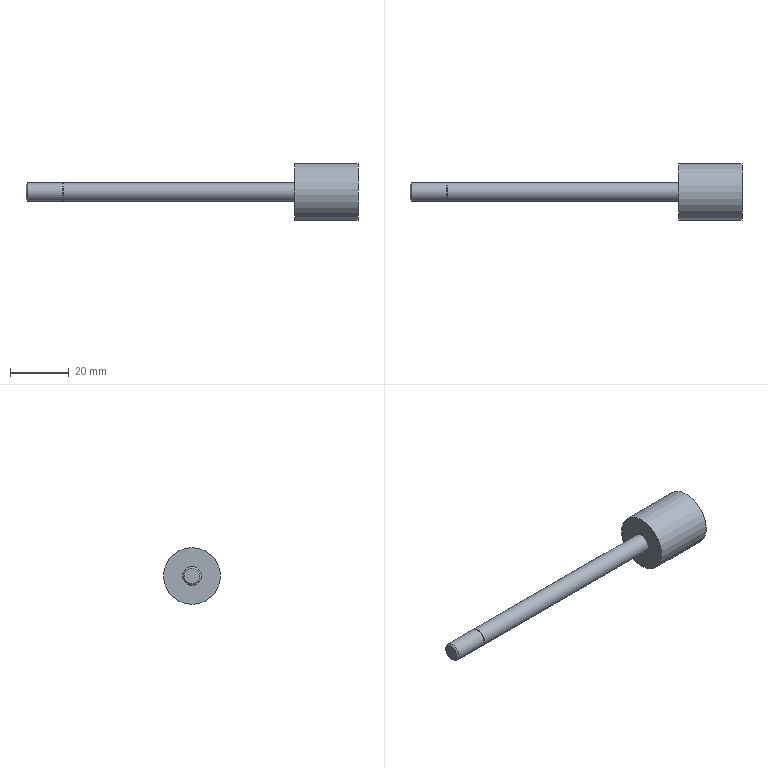Part | NX | features solid 2 | 1 solid | 10 faces | box 112.725 x 19.241 x 19.241 mm | volume 9120 mm3 | plane 5 | cylinder 4 | cone 1 | commonest cylinder face diameters 6.35 x2 5.842 x1 19.241 x1
STEP:
#1=CARTESIAN_POINT('',(78.588,0.,3.175));
#2=VERTEX_POINT('',#1);
#3=CARTESIAN_POINT('',(78.588,0.,0.));
#4=DIRECTION('',(-1.,0.,0.));
#5=DIRECTION('',(0.,0.,1.));
#6=AXIS2_PLACEMENT_3D('',#3,#4,#5);
#7=CIRCLE('',#6,3.175);
#8=EDGE_CURVE('',#2,#2,#7,.T.);
#9=ORIENTED_EDGE('',*,*,#8,.T.);
#10=EDGE_LOOP('',(#9));
#11=FACE_BOUND('',#10,.T.);
#12=CARTESIAN_POINT('',(0.,0.,3.175));
#13=VERTEX_POINT('',#12);
#14=CARTESIAN_POINT('',(0.,0.,0.));
#15=DIRECTION('',(-1.,0.,0.));
#16=DIRECTION('',(0.,0.,1.));
#17=AXIS2_PLACEMENT_3D('',#14,#15,#16);
#18=CIRCLE('',#17,3.175);
#19=EDGE_CURVE('',#13,#13,#18,.F.);
#20=ORIENTED_EDGE('',*,*,#19,.T.);
#21=EDGE_LOOP('',(#20));
#22=FACE_BOUND('',#21,.T.);
#23=CARTESIAN_POINT('',(100.025,0.,0.));
#24=DIRECTION('',(-1.,0.,0.));
#25=DIRECTION('',(0.,0.,1.));
#26=AXIS2_PLACEMENT_3D('',#23,#24,#25);
#27=CYLINDRICAL_SURFACE('',#26,3.175);
#28=ADVANCED_FACE('',(#11,#22),#27,.T.);
#29=CARTESIAN_POINT('',(78.588,0.,9.62));
#30=VERTEX_POINT('',#29);
#31=CARTESIAN_POINT('',(78.588,0.,0.));
#32=DIRECTION('',(-1.,0.,0.));
#33=DIRECTION('',(0.,0.,1.));
#34=AXIS2_PLACEMENT_3D('',#31,#32,#33);
#35=CIRCLE('',#34,9.62);
#36=EDGE_CURVE('',#30,#30,#35,.T.);
#37=ORIENTED_EDGE('',*,*,#36,.T.);
#38=EDGE_LOOP('',(#37));
#39=FACE_BOUND('',#38,.T.);
#40=ORIENTED_EDGE('',*,*,#8,.F.);
#41=EDGE_LOOP('',(#40));
#42=FACE_BOUND('',#41,.T.);
#43=CARTESIAN_POINT('',(78.588,3.175,0.));
#44=DIRECTION('',(-1.,0.,0.));
#45=DIRECTION('',(0.,0.,1.));
#46=AXIS2_PLACEMENT_3D('',#43,#44,#45);
#47=PLANE('',#46);
#48=ADVANCED_FACE('',(#39,#42),#47,.T.);
#49=CARTESIAN_POINT('',(100.025,0.,9.62));
#50=VERTEX_POINT('',#49);
#51=CARTESIAN_POINT('',(100.025,0.,0.));
#52=DIRECTION('',(-1.,0.,0.));
#53=DIRECTION('',(0.,0.,1.));
#54=AXIS2_PLACEMENT_3D('',#51,#52,#53);
#55=CIRCLE('',#54,9.62);
#56=EDGE_CURVE('',#50,#50,#55,.T.);
#57=ORIENTED_EDGE('',*,*,#56,.T.);
#58=EDGE_LOOP('',(#57));
#59=FACE_BOUND('',#58,.T.);
#60=ORIENTED_EDGE('',*,*,#36,.F.);
#61=EDGE_LOOP('',(#60));
#62=FACE_BOUND('',#61,.T.);
#63=CARTESIAN_POINT('',(100.025,0.,0.));
#64=DIRECTION('',(-1.,0.,0.));
#65=DIRECTION('',(0.,0.,1.));
#66=AXIS2_PLACEMENT_3D('',#63,#64,#65);
#67=CYLINDRICAL_SURFACE('',#66,9.62);
#68=ADVANCED_FACE('',(#59,#62),#67,.T.);
#69=ORIENTED_EDGE('',*,*,#56,.F.);
#70=EDGE_LOOP('',(#69));
#71=FACE_BOUND('',#70,.T.);
#72=CARTESIAN_POINT('',(100.025,9.62,0.));
#73=DIRECTION('',(1.,0.,0.));
#74=DIRECTION('',(0.,0.,-1.));
#75=AXIS2_PLACEMENT_3D('',#72,#73,#74);
#76=PLANE('',#75);
#77=ADVANCED_FACE('',(#71),#76,.T.);
#78=CARTESIAN_POINT('',(-0.254,0.,-3.175));
#79=VERTEX_POINT('',#78);
#80=CARTESIAN_POINT('',(-0.254,0.,0.));
#81=DIRECTION('',(1.,0.,0.));
#82=DIRECTION('',(0.,0.,-1.));
#83=AXIS2_PLACEMENT_3D('',#80,#81,#82);
#84=CIRCLE('',#83,3.175);
#85=EDGE_CURVE('',#79,#79,#84,.F.);
#86=ORIENTED_EDGE('',*,*,#85,.F.);
#87=EDGE_LOOP('',(#86));
#88=FACE_BOUND('',#87,.T.);
#89=CARTESIAN_POINT('',(-0.254,0.,2.921));
#90=VERTEX_POINT('',#89);
#91=CARTESIAN_POINT('',(-0.254,0.,0.));
#92=DIRECTION('',(-1.,0.,0.));
#93=DIRECTION('',(0.,0.,1.));
#94=AXIS2_PLACEMENT_3D('',#91,#92,#93);
#95=CIRCLE('',#94,2.921);
#96=EDGE_CURVE('',#90,#90,#95,.T.);
#97=ORIENTED_EDGE('',*,*,#96,.T.);
#98=EDGE_LOOP('',(#97));
#99=FACE_BOUND('',#98,.T.);
#100=CARTESIAN_POINT('',(-0.254,3.429,0.));
#101=DIRECTION('',(1.,0.,0.));
#102=DIRECTION('',(0.,0.,-1.));
#103=AXIS2_PLACEMENT_3D('',#100,#101,#102);
#104=PLANE('',#103);
#105=ADVANCED_FACE('',(#88,#99),#104,.T.);
#106=CARTESIAN_POINT('',(0.,0.,2.921));
#107=VERTEX_POINT('',#106);
#108=CARTESIAN_POINT('',(0.,0.,0.));
#109=DIRECTION('',(-1.,0.,0.));
#110=DIRECTION('',(0.,0.,1.));
#111=AXIS2_PLACEMENT_3D('',#108,#109,#110);
#112=CIRCLE('',#111,2.921);
#113=EDGE_CURVE('',#107,#107,#112,.T.);
#114=ORIENTED_EDGE('',*,*,#113,.T.);
#115=EDGE_LOOP('',(#114));
#116=FACE_BOUND('',#115,.T.);
#117=ORIENTED_EDGE('',*,*,#96,.F.);
#118=EDGE_LOOP('',(#117));
#119=FACE_BOUND('',#118,.T.);
#120=CARTESIAN_POINT('',(0.,0.,0.));
#121=DIRECTION('',(-1.,0.,0.));
#122=DIRECTION('',(0.,0.,1.));
#123=AXIS2_PLACEMENT_3D('',#120,#121,#122);
#124=CYLINDRICAL_SURFACE('',#123,2.921);
#125=ADVANCED_FACE('',(#116,#119),#124,.T.);
#126=ORIENTED_EDGE('',*,*,#19,.F.);
#127=EDGE_LOOP('',(#126));
#128=FACE_BOUND('',#127,.T.);
#129=ORIENTED_EDGE('',*,*,#113,.F.);
#130=EDGE_LOOP('',(#129));
#131=FACE_BOUND('',#130,.T.);
#132=CARTESIAN_POINT('',(0.,2.921,0.));
#133=DIRECTION('',(-1.,0.,0.));
#134=DIRECTION('',(0.,0.,1.));
#135=AXIS2_PLACEMENT_3D('',#132,#133,#134);
#136=PLANE('',#135);
#137=ADVANCED_FACE('',(#128,#131),#136,.T.);
#138=CARTESIAN_POINT('',(-12.7,0.,2.634));
#139=VERTEX_POINT('',#138);
#140=CARTESIAN_POINT('',(-12.7,0.,0.));
#141=DIRECTION('',(-1.,0.,0.));
#142=DIRECTION('',(0.,0.,1.));
#143=AXIS2_PLACEMENT_3D('',#140,#141,#142);
#144=CIRCLE('',#143,2.634);
#145=EDGE_CURVE('',#139,#139,#144,.T.);
#146=ORIENTED_EDGE('',*,*,#145,.T.);
#147=EDGE_LOOP('',(#146));
#148=FACE_BOUND('',#147,.T.);
#149=CARTESIAN_POINT('',(-12.7,0.,0.));
#150=DIRECTION('',(-1.,0.,0.));
#151=DIRECTION('',(0.,0.,1.));
#152=AXIS2_PLACEMENT_3D('',#149,#150,#151);
#153=PLANE('',#152);
#154=ADVANCED_FACE('',(#148),#153,.T.);
#155=CARTESIAN_POINT('',(-12.159,0.,3.175));
#156=VERTEX_POINT('',#155);
#157=CARTESIAN_POINT('',(-12.159,0.,0.));
#158=DIRECTION('',(-1.,0.,0.));
#159=DIRECTION('',(0.,0.,1.));
#160=AXIS2_PLACEMENT_3D('',#157,#158,#159);
#161=CIRCLE('',#160,3.175);
#162=EDGE_CURVE('',#156,#156,#161,.T.);
#163=ORIENTED_EDGE('',*,*,#162,.T.);
#164=EDGE_LOOP('',(#163));
#165=FACE_BOUND('',#164,.T.);
#166=ORIENTED_EDGE('',*,*,#145,.F.);
#167=EDGE_LOOP('',(#166));
#168=FACE_BOUND('',#167,.T.);
#169=CARTESIAN_POINT('',(-12.7,0.,0.));
#170=DIRECTION('',(1.,0.,0.));
#171=DIRECTION('',(0.,0.,-1.));
#172=AXIS2_PLACEMENT_3D('',#169,#170,#171);
#173=CONICAL_SURFACE('',#172,2.634,0.7854);
#174=ADVANCED_FACE('',(#165,#168),#173,.T.);
#175=ORIENTED_EDGE('',*,*,#162,.F.);
#176=EDGE_LOOP('',(#175));
#177=FACE_BOUND('',#176,.T.);
#178=ORIENTED_EDGE('',*,*,#85,.T.);
#179=EDGE_LOOP('',(#178));
#180=FACE_BOUND('',#179,.T.);
#181=CARTESIAN_POINT('',(100.025,0.,0.));
#182=DIRECTION('',(-1.,0.,0.));
#183=DIRECTION('',(0.,0.,1.));
#184=AXIS2_PLACEMENT_3D('',#181,#182,#183);
#185=CYLINDRICAL_SURFACE('',#184,3.175);
#186=ADVANCED_FACE('',(#177,#180),#185,.T.);
#187=CLOSED_SHELL('',(#28,#48,#68,#77,#105,#125,#137,#154,#174,#186));
#188=MANIFOLD_SOLID_BREP('',#187);
#189=(LENGTH_UNIT()NAMED_UNIT(*)SI_UNIT(.MILLI.,.METRE.));
#190=UNCERTAINTY_MEASURE_WITH_UNIT(LENGTH_MEASURE(0.00001),#189,'','');
#191=(NAMED_UNIT(*)PLANE_ANGLE_UNIT()SI_UNIT($,.RADIAN.));
#192=(NAMED_UNIT(*)SI_UNIT($,.STERADIAN.)SOLID_ANGLE_UNIT());
#193=(GEOMETRIC_REPRESENTATION_CONTEXT(3)GLOBAL_UNCERTAINTY_ASSIGNED_CONTEXT((#190))GLOBAL_UNIT_ASSIGNED_CONTEXT((#189,#191,#192))REPRESENTATION_CONTEXT('',''));
#194=ADVANCED_BREP_SHAPE_REPRESENTATION('',(#188),#193);